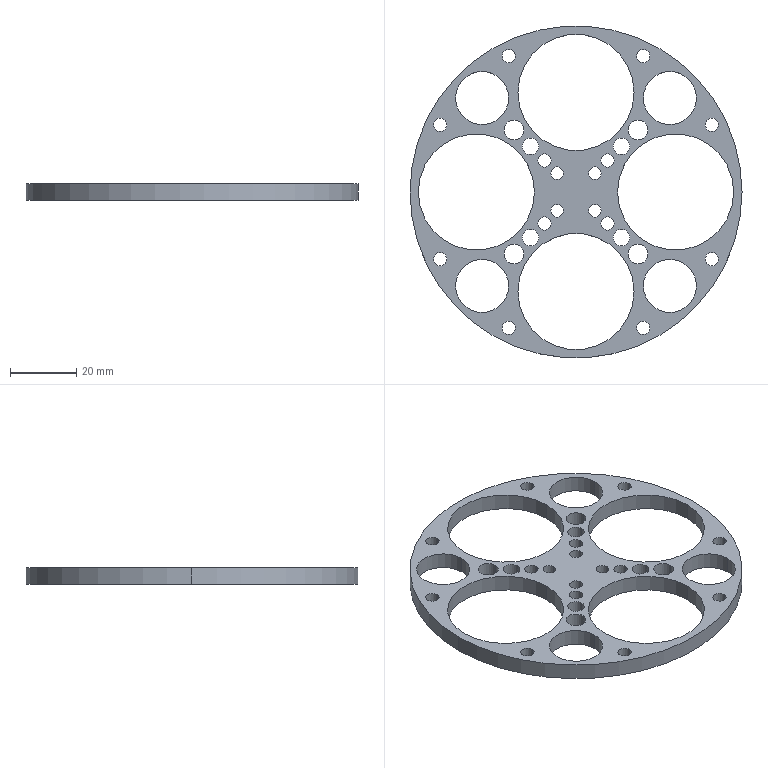Part | SolidWorks | features CirPattern 3, ICE 3, Extrusion 1 | 1 solid | 68 faces | box 100 x 100 x 5 mm | volume 14067 mm3 | cylinder 66 | plane 2 | commonest cylinder face diameters 4 x24 3.8 x8 5 x8 6 x8 16 x8 35 x8